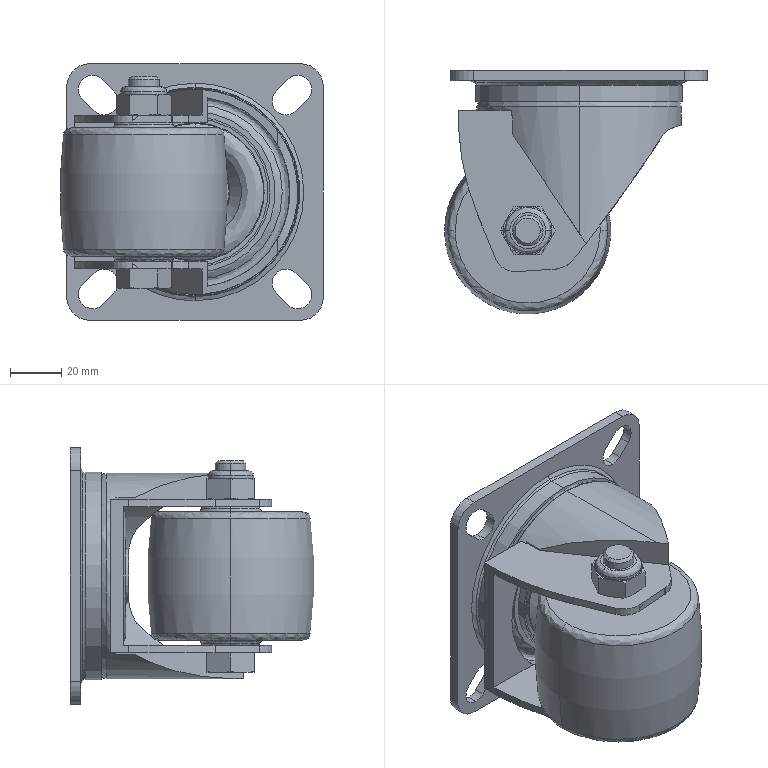Part | SolidWorks | features BaseBody 4 | 4 solids | 250 faces | box 102.5 x 95 x 100 mm | volume 269431 mm3 | spline 81 | plane 80 | cylinder 67 | cone 18 | torus 4 | commonest cylinder face diameters 11 x12 12 x6 18 x6 12.2 x4 20 x4 78.5 x4